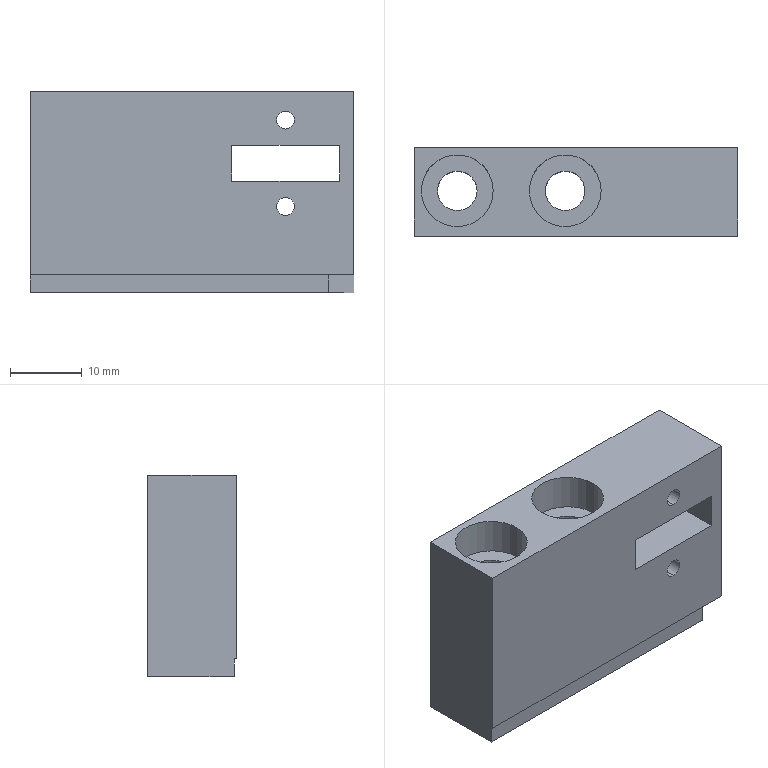Part | STEP file | detection side block right | 1 solid | 27 faces | box 45 x 12.3 x 28 mm | volume 12527 mm3 | plane 15 | cylinder 12 | commonest cylinder face diameters 2.5 x4 5.5 x4 10 x4